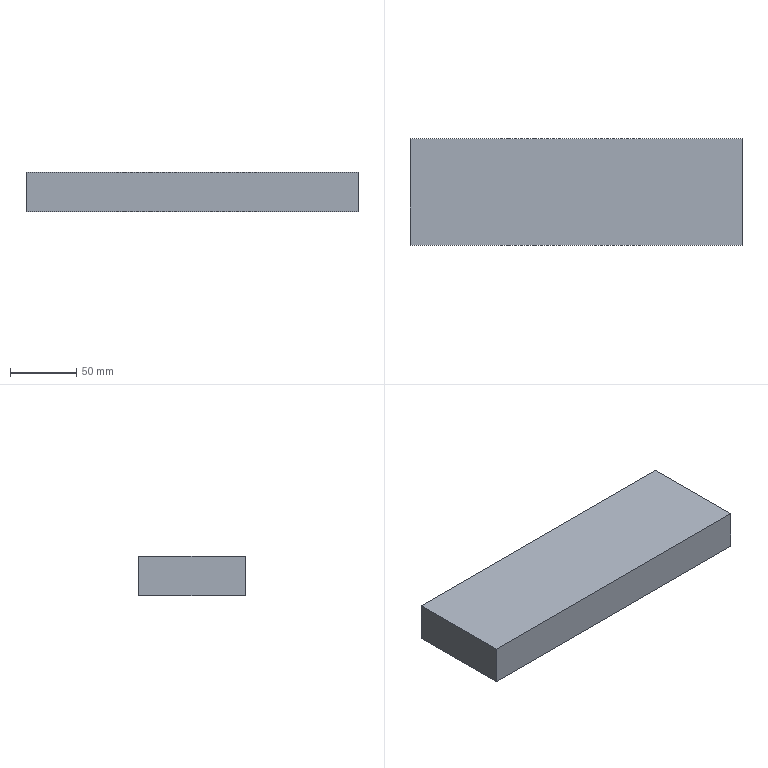Part | NX | features Part2 2 | 1 solid | 6 faces | box 250 x 80 x 30 mm | volume 600000 mm3 | plane 6
STEP:
#1=CARTESIAN_POINT('',(-125.,-40.,0.));
#2=VERTEX_POINT('',#1);
#3=CARTESIAN_POINT('',(-125.,40.,0.));
#4=VERTEX_POINT('',#3);
#5=CARTESIAN_POINT('',(-125.,-40.,0.));
#6=DIRECTION('',(0.,1.,0.));
#7=VECTOR('',#6,1000.);
#8=LINE('',#5,#7);
#9=EDGE_CURVE('',#2,#4,#8,.T.);
#10=ORIENTED_EDGE('',*,*,#9,.T.);
#11=CARTESIAN_POINT('',(125.,40.,0.));
#12=VERTEX_POINT('',#11);
#13=CARTESIAN_POINT('',(-125.,40.,0.));
#14=DIRECTION('',(1.,0.,0.));
#15=VECTOR('',#14,1000.);
#16=LINE('',#13,#15);
#17=EDGE_CURVE('',#4,#12,#16,.T.);
#18=ORIENTED_EDGE('',*,*,#17,.T.);
#19=CARTESIAN_POINT('',(125.,-40.,0.));
#20=VERTEX_POINT('',#19);
#21=CARTESIAN_POINT('',(125.,-40.,0.));
#22=DIRECTION('',(0.,1.,0.));
#23=VECTOR('',#22,1000.);
#24=LINE('',#21,#23);
#25=EDGE_CURVE('',#12,#20,#24,.F.);
#26=ORIENTED_EDGE('',*,*,#25,.T.);
#27=CARTESIAN_POINT('',(-125.,-40.,0.));
#28=DIRECTION('',(1.,0.,0.));
#29=VECTOR('',#28,1000.);
#30=LINE('',#27,#29);
#31=EDGE_CURVE('',#20,#2,#30,.F.);
#32=ORIENTED_EDGE('',*,*,#31,.T.);
#33=EDGE_LOOP('',(#10,#18,#26,#32));
#34=FACE_BOUND('',#33,.T.);
#35=CARTESIAN_POINT('',(125.,40.,0.));
#36=DIRECTION('',(0.,0.,-1.));
#37=DIRECTION('',(-1.,0.,0.));
#38=AXIS2_PLACEMENT_3D('',#35,#36,#37);
#39=PLANE('',#38);
#40=ADVANCED_FACE('',(#34),#39,.T.);
#41=CARTESIAN_POINT('',(125.,-40.,30.));
#42=VERTEX_POINT('',#41);
#43=CARTESIAN_POINT('',(125.,-40.,30.));
#44=DIRECTION('',(0.,0.,1.));
#45=VECTOR('',#44,1000.);
#46=LINE('',#43,#45);
#47=EDGE_CURVE('',#20,#42,#46,.T.);
#48=ORIENTED_EDGE('',*,*,#47,.T.);
#49=CARTESIAN_POINT('',(-125.,-40.,30.));
#50=VERTEX_POINT('',#49);
#51=CARTESIAN_POINT('',(125.,-40.,30.));
#52=DIRECTION('',(-1.,0.,0.));
#53=VECTOR('',#52,1000.);
#54=LINE('',#51,#53);
#55=EDGE_CURVE('',#42,#50,#54,.T.);
#56=ORIENTED_EDGE('',*,*,#55,.T.);
#57=CARTESIAN_POINT('',(-125.,-40.,30.));
#58=DIRECTION('',(0.,0.,-1.));
#59=VECTOR('',#58,1000.);
#60=LINE('',#57,#59);
#61=EDGE_CURVE('',#50,#2,#60,.T.);
#62=ORIENTED_EDGE('',*,*,#61,.T.);
#63=ORIENTED_EDGE('',*,*,#31,.F.);
#64=EDGE_LOOP('',(#48,#56,#62,#63));
#65=FACE_BOUND('',#64,.T.);
#66=CARTESIAN_POINT('',(-125.,-40.,30.));
#67=DIRECTION('',(0.,1.,0.));
#68=DIRECTION('',(0.,0.,1.));
#69=AXIS2_PLACEMENT_3D('',#66,#67,#68);
#70=PLANE('',#69);
#71=ADVANCED_FACE('',(#65),#70,.F.);
#72=ORIENTED_EDGE('',*,*,#61,.F.);
#73=CARTESIAN_POINT('',(-125.,40.,30.));
#74=VERTEX_POINT('',#73);
#75=CARTESIAN_POINT('',(-125.,40.,30.));
#76=DIRECTION('',(0.,1.,0.));
#77=VECTOR('',#76,1000.);
#78=LINE('',#75,#77);
#79=EDGE_CURVE('',#50,#74,#78,.T.);
#80=ORIENTED_EDGE('',*,*,#79,.T.);
#81=CARTESIAN_POINT('',(-125.,40.,30.));
#82=DIRECTION('',(0.,0.,-1.));
#83=VECTOR('',#82,1000.);
#84=LINE('',#81,#83);
#85=EDGE_CURVE('',#74,#4,#84,.T.);
#86=ORIENTED_EDGE('',*,*,#85,.T.);
#87=ORIENTED_EDGE('',*,*,#9,.F.);
#88=EDGE_LOOP('',(#72,#80,#86,#87));
#89=FACE_BOUND('',#88,.T.);
#90=CARTESIAN_POINT('',(-125.,-40.,30.));
#91=DIRECTION('',(1.,0.,0.));
#92=DIRECTION('',(0.,0.,-1.));
#93=AXIS2_PLACEMENT_3D('',#90,#91,#92);
#94=PLANE('',#93);
#95=ADVANCED_FACE('',(#89),#94,.F.);
#96=ORIENTED_EDGE('',*,*,#85,.F.);
#97=CARTESIAN_POINT('',(125.,40.,30.));
#98=VERTEX_POINT('',#97);
#99=CARTESIAN_POINT('',(125.,40.,30.));
#100=DIRECTION('',(-1.,0.,0.));
#101=VECTOR('',#100,1000.);
#102=LINE('',#99,#101);
#103=EDGE_CURVE('',#74,#98,#102,.F.);
#104=ORIENTED_EDGE('',*,*,#103,.T.);
#105=CARTESIAN_POINT('',(125.,40.,30.));
#106=DIRECTION('',(0.,0.,1.));
#107=VECTOR('',#106,1000.);
#108=LINE('',#105,#107);
#109=EDGE_CURVE('',#98,#12,#108,.F.);
#110=ORIENTED_EDGE('',*,*,#109,.T.);
#111=ORIENTED_EDGE('',*,*,#17,.F.);
#112=EDGE_LOOP('',(#96,#104,#110,#111));
#113=FACE_BOUND('',#112,.T.);
#114=CARTESIAN_POINT('',(-125.,40.,30.));
#115=DIRECTION('',(0.,-1.,0.));
#116=DIRECTION('',(0.,0.,-1.));
#117=AXIS2_PLACEMENT_3D('',#114,#115,#116);
#118=PLANE('',#117);
#119=ADVANCED_FACE('',(#113),#118,.F.);
#120=ORIENTED_EDGE('',*,*,#109,.F.);
#121=CARTESIAN_POINT('',(125.,40.,30.));
#122=DIRECTION('',(0.,1.,0.));
#123=VECTOR('',#122,1000.);
#124=LINE('',#121,#123);
#125=EDGE_CURVE('',#98,#42,#124,.F.);
#126=ORIENTED_EDGE('',*,*,#125,.T.);
#127=ORIENTED_EDGE('',*,*,#47,.F.);
#128=ORIENTED_EDGE('',*,*,#25,.F.);
#129=EDGE_LOOP('',(#120,#126,#127,#128));
#130=FACE_BOUND('',#129,.T.);
#131=CARTESIAN_POINT('',(125.,-40.,30.));
#132=DIRECTION('',(-1.,0.,0.));
#133=DIRECTION('',(0.,0.,1.));
#134=AXIS2_PLACEMENT_3D('',#131,#132,#133);
#135=PLANE('',#134);
#136=ADVANCED_FACE('',(#130),#135,.F.);
#137=ORIENTED_EDGE('',*,*,#103,.F.);
#138=ORIENTED_EDGE('',*,*,#79,.F.);
#139=ORIENTED_EDGE('',*,*,#55,.F.);
#140=ORIENTED_EDGE('',*,*,#125,.F.);
#141=EDGE_LOOP('',(#137,#138,#139,#140));
#142=FACE_BOUND('',#141,.T.);
#143=CARTESIAN_POINT('',(125.,40.,30.));
#144=DIRECTION('',(0.,0.,-1.));
#145=DIRECTION('',(-1.,0.,0.));
#146=AXIS2_PLACEMENT_3D('',#143,#144,#145);
#147=PLANE('',#146);
#148=ADVANCED_FACE('',(#142),#147,.F.);
#149=CLOSED_SHELL('',(#40,#71,#95,#119,#136,#148));
#150=MANIFOLD_SOLID_BREP('',#149);
#151=(LENGTH_UNIT()NAMED_UNIT(*)SI_UNIT(.MILLI.,.METRE.));
#152=UNCERTAINTY_MEASURE_WITH_UNIT(LENGTH_MEASURE(0.00001),#151,'','');
#153=(NAMED_UNIT(*)PLANE_ANGLE_UNIT()SI_UNIT($,.RADIAN.));
#154=(NAMED_UNIT(*)SI_UNIT($,.STERADIAN.)SOLID_ANGLE_UNIT());
#155=(GEOMETRIC_REPRESENTATION_CONTEXT(3)GLOBAL_UNCERTAINTY_ASSIGNED_CONTEXT((#152))GLOBAL_UNIT_ASSIGNED_CONTEXT((#151,#153,#154))REPRESENTATION_CONTEXT('',''));
#156=ADVANCED_BREP_SHAPE_REPRESENTATION('',(#150),#155);